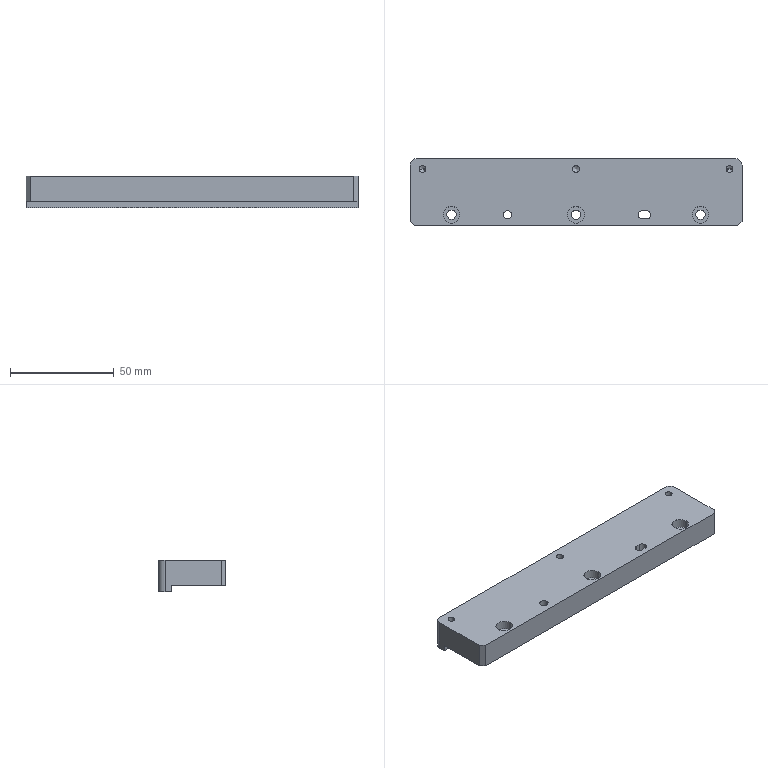Part | STEP file | QA-AD04 | 1 solid | 52 faces | box 160 x 32 x 15.1 mm | volume 62990 mm3 | cylinder 25 | plane 15 | cone 12 | commonest cylinder face diameters 3.3 x6 4.5 x6 8 x6 4 x5 6 x2